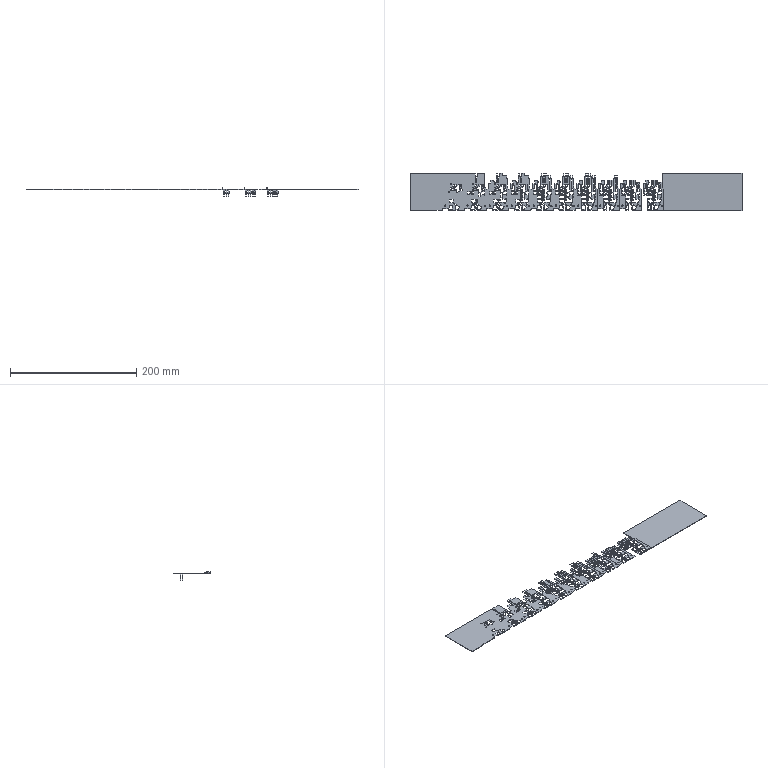Part | NX | features BREP 4 | 8 solids | 2473 faces | box 525 x 60 x 13.3 mm | volume 13484 mm3 | plane 1379 | cylinder 1094 | commonest cylinder face diameters 1 x1010 2 x22 2.2 x19 72.496 x11 188.049 x10 72.701 x8